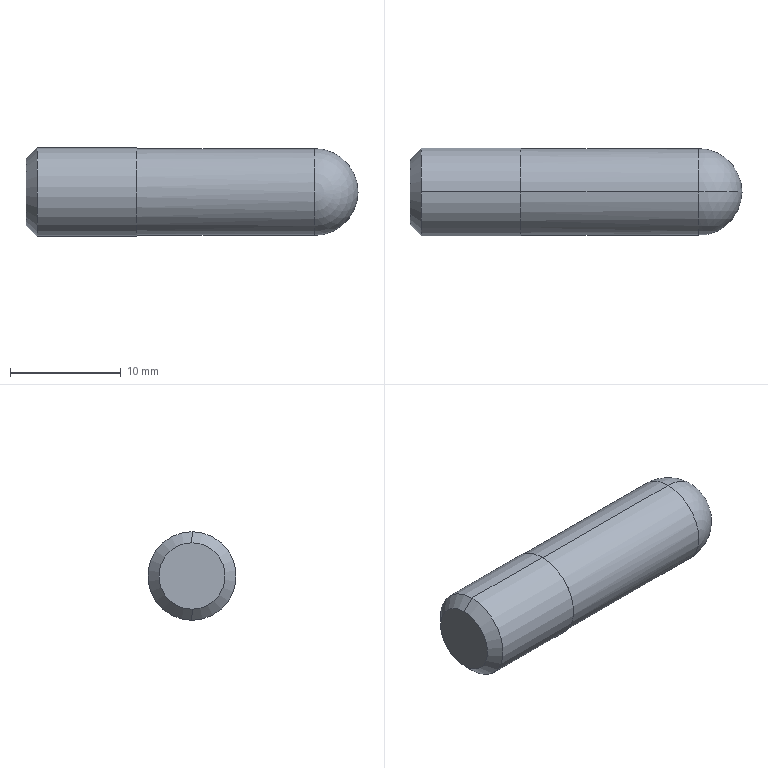Part | SolidWorks | features Chamfer 1, Extrusion 1, Fillet 1, ICE 1 | 1 solid | 10 faces | box 30 x 8 x 8 mm | volume 1396 mm3 | cylinder 4 | cone 2 | sphere 2 | plane 2 | commonest cylinder face diameters 7.85 x2 8 x2
STEP:
#1=CARTESIAN_POINT('',(0.,0.,3.));
#2=VERTEX_POINT('',#1);
#3=CARTESIAN_POINT('',(0.,0.,-3.));
#4=VERTEX_POINT('',#3);
#5=CARTESIAN_POINT('',(0.,0.,0.));
#6=DIRECTION('',(-1.,0.,0.));
#7=DIRECTION('',(0.,0.,-1.));
#8=AXIS2_PLACEMENT_3D('',#5,#6,#7);
#9=CIRCLE('',#8,3.);
#10=EDGE_CURVE('',#2,#4,#9,.T.);
#11=ORIENTED_EDGE('',*,*,#10,.F.);
#12=CARTESIAN_POINT('',(1.,0.,4.));
#13=VERTEX_POINT('',#12);
#14=CARTESIAN_POINT('',(1.,0.,4.));
#15=DIRECTION('',(0.7071,0.,0.7071));
#16=VECTOR('',#15,1000.);
#17=LINE('',#14,#16);
#18=EDGE_CURVE('',#2,#13,#17,.T.);
#19=ORIENTED_EDGE('',*,*,#18,.T.);
#20=CARTESIAN_POINT('',(1.,0.,-4.));
#21=VERTEX_POINT('',#20);
#22=CARTESIAN_POINT('',(1.,0.,0.));
#23=DIRECTION('',(1.,0.,0.));
#24=DIRECTION('',(0.,0.,-1.));
#25=AXIS2_PLACEMENT_3D('',#22,#23,#24);
#26=CIRCLE('',#25,4.);
#27=EDGE_CURVE('',#21,#13,#26,.T.);
#28=ORIENTED_EDGE('',*,*,#27,.F.);
#29=CARTESIAN_POINT('',(1.,0.,-4.));
#30=DIRECTION('',(0.7071,0.,-0.7071));
#31=VECTOR('',#30,1000.);
#32=LINE('',#29,#31);
#33=EDGE_CURVE('',#4,#21,#32,.T.);
#34=ORIENTED_EDGE('',*,*,#33,.F.);
#35=EDGE_LOOP('',(#11,#19,#28,#34));
#36=FACE_OUTER_BOUND('',#35,.T.);
#37=CARTESIAN_POINT('',(1.,0.,0.));
#38=DIRECTION('',(1.,0.,0.));
#39=DIRECTION('',(0.,0.,-1.));
#40=AXIS2_PLACEMENT_3D('',#37,#38,#39);
#41=CONICAL_SURFACE('',#40,4.,0.7854);
#42=ADVANCED_FACE('',(#36),#41,.T.);
#43=CARTESIAN_POINT('',(26.075,0.,3.925));
#44=VERTEX_POINT('',#43);
#45=CARTESIAN_POINT('',(26.075,0.,-3.925));
#46=VERTEX_POINT('',#45);
#47=CARTESIAN_POINT('',(26.075,0.,0.));
#48=DIRECTION('',(-1.,0.,0.));
#49=DIRECTION('',(0.,0.,1.));
#50=AXIS2_PLACEMENT_3D('',#47,#48,#49);
#51=CIRCLE('',#50,3.925);
#52=EDGE_CURVE('',#44,#46,#51,.T.);
#53=ORIENTED_EDGE('',*,*,#52,.F.);
#54=CARTESIAN_POINT('',(30.,0.,0.));
#55=VERTEX_POINT('',#54);
#56=CARTESIAN_POINT('',(26.075,0.,0.));
#57=DIRECTION('',(0.,1.,0.));
#58=DIRECTION('',(0.,0.,1.));
#59=AXIS2_PLACEMENT_3D('',#56,#57,#58);
#60=CIRCLE('',#59,3.925);
#61=EDGE_CURVE('',#44,#55,#60,.T.);
#62=ORIENTED_EDGE('',*,*,#61,.T.);
#63=CARTESIAN_POINT('',(26.075,0.,0.));
#64=DIRECTION('',(0.,-1.,0.));
#65=DIRECTION('',(0.,0.,-1.));
#66=AXIS2_PLACEMENT_3D('',#63,#64,#65);
#67=CIRCLE('',#66,3.925);
#68=EDGE_CURVE('',#46,#55,#67,.T.);
#69=ORIENTED_EDGE('',*,*,#68,.F.);
#70=EDGE_LOOP('',(#53,#62,#69));
#71=FACE_OUTER_BOUND('',#70,.T.);
#72=CARTESIAN_POINT('',(26.075,0.,0.));
#73=DIRECTION('',(0.,1.,0.));
#74=DIRECTION('',(0.,0.,-1.));
#75=AXIS2_PLACEMENT_3D('',#72,#73,#74);
#76=SPHERICAL_SURFACE('',#75,3.925);
#77=ADVANCED_FACE('',(#71),#76,.T.);
#78=ORIENTED_EDGE('',*,*,#52,.T.);
#79=CARTESIAN_POINT('',(10.,0.,-3.925));
#80=VERTEX_POINT('',#79);
#81=CARTESIAN_POINT('',(30.,0.,-3.925));
#82=DIRECTION('',(-1.,0.,0.));
#83=VECTOR('',#82,1000.);
#84=LINE('',#81,#83);
#85=EDGE_CURVE('',#46,#80,#84,.T.);
#86=ORIENTED_EDGE('',*,*,#85,.T.);
#87=CARTESIAN_POINT('',(10.,0.,3.925));
#88=VERTEX_POINT('',#87);
#89=CARTESIAN_POINT('',(10.,0.,0.));
#90=DIRECTION('',(1.,0.,0.));
#91=DIRECTION('',(0.,0.,-1.));
#92=AXIS2_PLACEMENT_3D('',#89,#90,#91);
#93=CIRCLE('',#92,3.925);
#94=EDGE_CURVE('',#80,#88,#93,.T.);
#95=ORIENTED_EDGE('',*,*,#94,.T.);
#96=CARTESIAN_POINT('',(30.,0.,3.925));
#97=DIRECTION('',(-1.,0.,0.));
#98=VECTOR('',#97,1000.);
#99=LINE('',#96,#98);
#100=EDGE_CURVE('',#44,#88,#99,.T.);
#101=ORIENTED_EDGE('',*,*,#100,.F.);
#102=EDGE_LOOP('',(#78,#86,#95,#101));
#103=FACE_OUTER_BOUND('',#102,.T.);
#104=CARTESIAN_POINT('',(30.,0.,0.));
#105=DIRECTION('',(-1.,0.,0.));
#106=DIRECTION('',(0.,0.,1.));
#107=AXIS2_PLACEMENT_3D('',#104,#105,#106);
#108=CYLINDRICAL_SURFACE('',#107,3.925);
#109=ADVANCED_FACE('',(#103),#108,.T.);
#110=CARTESIAN_POINT('',(10.,0.,-4.));
#111=VERTEX_POINT('',#110);
#112=CARTESIAN_POINT('',(10.,0.,4.));
#113=VERTEX_POINT('',#112);
#114=CARTESIAN_POINT('',(10.,0.,0.));
#115=DIRECTION('',(1.,0.,0.));
#116=DIRECTION('',(0.,0.,-1.));
#117=AXIS2_PLACEMENT_3D('',#114,#115,#116);
#118=CIRCLE('',#117,4.);
#119=EDGE_CURVE('',#111,#113,#118,.T.);
#120=ORIENTED_EDGE('',*,*,#119,.F.);
#121=CARTESIAN_POINT('',(10.,0.,-4.));
#122=DIRECTION('',(-1.,0.,0.));
#123=VECTOR('',#122,1000.);
#124=LINE('',#121,#123);
#125=EDGE_CURVE('',#111,#21,#124,.T.);
#126=ORIENTED_EDGE('',*,*,#125,.T.);
#127=ORIENTED_EDGE('',*,*,#27,.T.);
#128=CARTESIAN_POINT('',(10.,0.,4.));
#129=DIRECTION('',(-1.,0.,0.));
#130=VECTOR('',#129,1000.);
#131=LINE('',#128,#130);
#132=EDGE_CURVE('',#113,#13,#131,.T.);
#133=ORIENTED_EDGE('',*,*,#132,.F.);
#134=EDGE_LOOP('',(#120,#126,#127,#133));
#135=FACE_OUTER_BOUND('',#134,.T.);
#136=CARTESIAN_POINT('',(10.,0.,0.));
#137=DIRECTION('',(-1.,0.,0.));
#138=DIRECTION('',(0.,0.,1.));
#139=AXIS2_PLACEMENT_3D('',#136,#137,#138);
#140=CYLINDRICAL_SURFACE('',#139,4.);
#141=ADVANCED_FACE('',(#135),#140,.T.);
#142=ORIENTED_EDGE('',*,*,#125,.F.);
#143=CARTESIAN_POINT('',(10.,0.,0.));
#144=DIRECTION('',(1.,0.,0.));
#145=DIRECTION('',(0.,0.,-1.));
#146=AXIS2_PLACEMENT_3D('',#143,#144,#145);
#147=CIRCLE('',#146,4.);
#148=EDGE_CURVE('',#113,#111,#147,.T.);
#149=ORIENTED_EDGE('',*,*,#148,.F.);
#150=ORIENTED_EDGE('',*,*,#132,.T.);
#151=CARTESIAN_POINT('',(1.,0.,0.));
#152=DIRECTION('',(1.,0.,0.));
#153=DIRECTION('',(0.,0.,-1.));
#154=AXIS2_PLACEMENT_3D('',#151,#152,#153);
#155=CIRCLE('',#154,4.);
#156=EDGE_CURVE('',#13,#21,#155,.T.);
#157=ORIENTED_EDGE('',*,*,#156,.T.);
#158=EDGE_LOOP('',(#142,#149,#150,#157));
#159=FACE_OUTER_BOUND('',#158,.T.);
#160=CARTESIAN_POINT('',(10.,0.,0.));
#161=DIRECTION('',(-1.,0.,0.));
#162=DIRECTION('',(0.,0.,1.));
#163=AXIS2_PLACEMENT_3D('',#160,#161,#162);
#164=CYLINDRICAL_SURFACE('',#163,4.);
#165=ADVANCED_FACE('',(#159),#164,.T.);
#166=CARTESIAN_POINT('',(10.,0.,0.));
#167=DIRECTION('',(1.,0.,0.));
#168=DIRECTION('',(0.,0.,-1.));
#169=AXIS2_PLACEMENT_3D('',#166,#167,#168);
#170=CIRCLE('',#169,3.925);
#171=EDGE_CURVE('',#88,#80,#170,.T.);
#172=ORIENTED_EDGE('',*,*,#171,.F.);
#173=ORIENTED_EDGE('',*,*,#94,.F.);
#174=EDGE_LOOP('',(#172,#173));
#175=FACE_BOUND('',#174,.T.);
#176=ORIENTED_EDGE('',*,*,#148,.T.);
#177=ORIENTED_EDGE('',*,*,#119,.T.);
#178=EDGE_LOOP('',(#176,#177));
#179=FACE_OUTER_BOUND('',#178,.T.);
#180=CARTESIAN_POINT('',(10.,0.,0.));
#181=DIRECTION('',(1.,0.,0.));
#182=DIRECTION('',(0.,0.,-1.));
#183=AXIS2_PLACEMENT_3D('',#180,#181,#182);
#184=PLANE('',#183);
#185=ADVANCED_FACE('',(#175,#179),#184,.T.);
#186=CARTESIAN_POINT('',(0.,0.,0.));
#187=DIRECTION('',(-1.,0.,0.));
#188=DIRECTION('',(0.,0.,-1.));
#189=AXIS2_PLACEMENT_3D('',#186,#187,#188);
#190=CIRCLE('',#189,3.);
#191=EDGE_CURVE('',#4,#2,#190,.T.);
#192=ORIENTED_EDGE('',*,*,#191,.T.);
#193=ORIENTED_EDGE('',*,*,#10,.T.);
#194=EDGE_LOOP('',(#192,#193));
#195=FACE_OUTER_BOUND('',#194,.T.);
#196=CARTESIAN_POINT('',(0.,0.,0.));
#197=DIRECTION('',(1.,0.,0.));
#198=DIRECTION('',(0.,0.,-1.));
#199=AXIS2_PLACEMENT_3D('',#196,#197,#198);
#200=PLANE('',#199);
#201=ADVANCED_FACE('',(#195),#200,.F.);
#202=ORIENTED_EDGE('',*,*,#85,.F.);
#203=CARTESIAN_POINT('',(26.075,0.,0.));
#204=DIRECTION('',(-1.,0.,0.));
#205=DIRECTION('',(0.,0.,1.));
#206=AXIS2_PLACEMENT_3D('',#203,#204,#205);
#207=CIRCLE('',#206,3.925);
#208=EDGE_CURVE('',#46,#44,#207,.T.);
#209=ORIENTED_EDGE('',*,*,#208,.T.);
#210=ORIENTED_EDGE('',*,*,#100,.T.);
#211=ORIENTED_EDGE('',*,*,#171,.T.);
#212=EDGE_LOOP('',(#202,#209,#210,#211));
#213=FACE_OUTER_BOUND('',#212,.T.);
#214=CARTESIAN_POINT('',(30.,0.,0.));
#215=DIRECTION('',(-1.,0.,0.));
#216=DIRECTION('',(0.,0.,1.));
#217=AXIS2_PLACEMENT_3D('',#214,#215,#216);
#218=CYLINDRICAL_SURFACE('',#217,3.925);
#219=ADVANCED_FACE('',(#213),#218,.T.);
#220=ORIENTED_EDGE('',*,*,#61,.F.);
#221=ORIENTED_EDGE('',*,*,#208,.F.);
#222=ORIENTED_EDGE('',*,*,#68,.T.);
#223=EDGE_LOOP('',(#220,#221,#222));
#224=FACE_OUTER_BOUND('',#223,.T.);
#225=CARTESIAN_POINT('',(26.075,0.,0.));
#226=DIRECTION('',(0.,1.,0.));
#227=DIRECTION('',(0.,0.,-1.));
#228=AXIS2_PLACEMENT_3D('',#225,#226,#227);
#229=SPHERICAL_SURFACE('',#228,3.925);
#230=ADVANCED_FACE('',(#224),#229,.T.);
#231=ORIENTED_EDGE('',*,*,#18,.F.);
#232=ORIENTED_EDGE('',*,*,#191,.F.);
#233=ORIENTED_EDGE('',*,*,#33,.T.);
#234=ORIENTED_EDGE('',*,*,#156,.F.);
#235=EDGE_LOOP('',(#231,#232,#233,#234));
#236=FACE_OUTER_BOUND('',#235,.T.);
#237=CARTESIAN_POINT('',(1.,0.,0.));
#238=DIRECTION('',(1.,0.,0.));
#239=DIRECTION('',(0.,0.,-1.));
#240=AXIS2_PLACEMENT_3D('',#237,#238,#239);
#241=CONICAL_SURFACE('',#240,4.,0.7854);
#242=ADVANCED_FACE('',(#236),#241,.T.);
#243=CLOSED_SHELL('',(#42,#77,#109,#141,#165,#185,#201,#219,#230,#242));
#244=MANIFOLD_SOLID_BREP('',#243);
#245=CARTESIAN_POINT('',(0.,0.,0.));
#246=DIRECTION('',(0.,0.,1.));
#247=DIRECTION('',(1.,0.,0.));
#248=AXIS2_PLACEMENT_3D('',#245,#246,#247);
#249=(LENGTH_UNIT()NAMED_UNIT(*)SI_UNIT(.MILLI.,.METRE.));
#250=UNCERTAINTY_MEASURE_WITH_UNIT(LENGTH_MEASURE(0.00001),#249,'','');
#251=(NAMED_UNIT(*)PLANE_ANGLE_UNIT()SI_UNIT($,.RADIAN.));
#252=(NAMED_UNIT(*)SI_UNIT($,.STERADIAN.)SOLID_ANGLE_UNIT());
#253=(GEOMETRIC_REPRESENTATION_CONTEXT(3)GLOBAL_UNCERTAINTY_ASSIGNED_CONTEXT((#250))GLOBAL_UNIT_ASSIGNED_CONTEXT((#249,#251,#252))REPRESENTATION_CONTEXT('',''));
#254=ADVANCED_BREP_SHAPE_REPRESENTATION('',(#244,#248),#253);